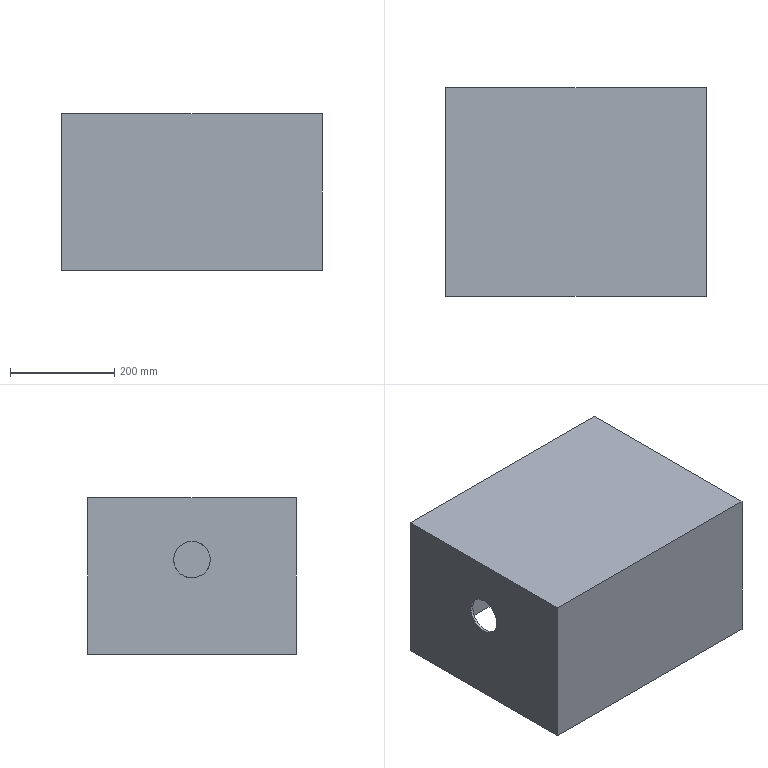Part | NX | features DATUM_CSYS 2, BLOCK 1, EXTRUDE 1, SHELL 1, SKETCH 1 | 1 solid | 12 faces | box 500 x 400 x 300 mm | volume 3606133 mm3 | plane 11 | cylinder 1 | commonest cylinder face diameters 70.226 x1
STEP:
#1=CARTESIAN_POINT('',(500.,0.,0.));
#2=VERTEX_POINT('',#1);
#3=CARTESIAN_POINT('',(500.,400.,0.));
#4=VERTEX_POINT('',#3);
#5=CARTESIAN_POINT('',(500.,200.,0.));
#6=DIRECTION('',(0.,1.,0.));
#7=VECTOR('',#6,1000.);
#8=LINE('',#5,#7);
#9=EDGE_CURVE('',#2,#4,#8,.T.);
#10=ORIENTED_EDGE('',*,*,#9,.F.);
#11=CARTESIAN_POINT('',(0.,0.,0.));
#12=VERTEX_POINT('',#11);
#13=CARTESIAN_POINT('',(250.,0.,0.));
#14=DIRECTION('',(1.,0.,0.));
#15=VECTOR('',#14,1000.);
#16=LINE('',#13,#15);
#17=EDGE_CURVE('',#12,#2,#16,.T.);
#18=ORIENTED_EDGE('',*,*,#17,.F.);
#19=CARTESIAN_POINT('',(0.,400.,0.));
#20=VERTEX_POINT('',#19);
#21=CARTESIAN_POINT('',(0.,200.,0.));
#22=DIRECTION('',(0.,-1.,0.));
#23=VECTOR('',#22,1000.);
#24=LINE('',#21,#23);
#25=EDGE_CURVE('',#20,#12,#24,.T.);
#26=ORIENTED_EDGE('',*,*,#25,.F.);
#27=CARTESIAN_POINT('',(250.,400.,0.));
#28=DIRECTION('',(-1.,0.,0.));
#29=VECTOR('',#28,1000.);
#30=LINE('',#27,#29);
#31=EDGE_CURVE('',#4,#20,#30,.T.);
#32=ORIENTED_EDGE('',*,*,#31,.F.);
#33=EDGE_LOOP('',(#10,#18,#26,#32));
#34=FACE_BOUND('',#33,.T.);
#35=CARTESIAN_POINT('',(5.,5.,0.));
#36=VERTEX_POINT('',#35);
#37=CARTESIAN_POINT('',(495.,5.,0.));
#38=VERTEX_POINT('',#37);
#39=CARTESIAN_POINT('',(250.,5.,0.));
#40=DIRECTION('',(1.,0.,0.));
#41=VECTOR('',#40,1000.);
#42=LINE('',#39,#41);
#43=EDGE_CURVE('',#36,#38,#42,.T.);
#44=ORIENTED_EDGE('',*,*,#43,.T.);
#45=CARTESIAN_POINT('',(495.,395.,0.));
#46=VERTEX_POINT('',#45);
#47=CARTESIAN_POINT('',(495.,200.,0.));
#48=DIRECTION('',(0.,1.,0.));
#49=VECTOR('',#48,1000.);
#50=LINE('',#47,#49);
#51=EDGE_CURVE('',#38,#46,#50,.T.);
#52=ORIENTED_EDGE('',*,*,#51,.T.);
#53=CARTESIAN_POINT('',(5.,395.,0.));
#54=VERTEX_POINT('',#53);
#55=CARTESIAN_POINT('',(250.,395.,0.));
#56=DIRECTION('',(-1.,0.,0.));
#57=VECTOR('',#56,1000.);
#58=LINE('',#55,#57);
#59=EDGE_CURVE('',#46,#54,#58,.T.);
#60=ORIENTED_EDGE('',*,*,#59,.T.);
#61=CARTESIAN_POINT('',(5.,200.,0.));
#62=DIRECTION('',(0.,-1.,0.));
#63=VECTOR('',#62,1000.);
#64=LINE('',#61,#63);
#65=EDGE_CURVE('',#54,#36,#64,.T.);
#66=ORIENTED_EDGE('',*,*,#65,.T.);
#67=EDGE_LOOP('',(#44,#52,#60,#66));
#68=FACE_BOUND('',#67,.T.);
#69=CARTESIAN_POINT('',(250.,200.,0.));
#70=DIRECTION('',(0.,0.,-1.));
#71=DIRECTION('',(-1.,0.,0.));
#72=AXIS2_PLACEMENT_3D('',#69,#70,#71);
#73=PLANE('',#72);
#74=ADVANCED_FACE('',(#34,#68),#73,.T.);
#75=CARTESIAN_POINT('',(500.,0.,300.));
#76=VERTEX_POINT('',#75);
#77=CARTESIAN_POINT('',(0.,0.,300.));
#78=VERTEX_POINT('',#77);
#79=CARTESIAN_POINT('',(250.,0.,300.));
#80=DIRECTION('',(-1.,0.,0.));
#81=VECTOR('',#80,1000.);
#82=LINE('',#79,#81);
#83=EDGE_CURVE('',#76,#78,#82,.T.);
#84=ORIENTED_EDGE('',*,*,#83,.F.);
#85=CARTESIAN_POINT('',(500.,400.,300.));
#86=VERTEX_POINT('',#85);
#87=CARTESIAN_POINT('',(500.,200.,300.));
#88=DIRECTION('',(0.,-1.,0.));
#89=VECTOR('',#88,1000.);
#90=LINE('',#87,#89);
#91=EDGE_CURVE('',#86,#76,#90,.T.);
#92=ORIENTED_EDGE('',*,*,#91,.F.);
#93=CARTESIAN_POINT('',(0.,400.,300.));
#94=VERTEX_POINT('',#93);
#95=CARTESIAN_POINT('',(250.,400.,300.));
#96=DIRECTION('',(1.,0.,0.));
#97=VECTOR('',#96,1000.);
#98=LINE('',#95,#97);
#99=EDGE_CURVE('',#94,#86,#98,.T.);
#100=ORIENTED_EDGE('',*,*,#99,.F.);
#101=CARTESIAN_POINT('',(0.,200.,300.));
#102=DIRECTION('',(0.,1.,0.));
#103=VECTOR('',#102,1000.);
#104=LINE('',#101,#103);
#105=EDGE_CURVE('',#78,#94,#104,.T.);
#106=ORIENTED_EDGE('',*,*,#105,.F.);
#107=EDGE_LOOP('',(#84,#92,#100,#106));
#108=FACE_BOUND('',#107,.T.);
#109=CARTESIAN_POINT('',(250.,200.,300.));
#110=DIRECTION('',(0.,0.,1.));
#111=DIRECTION('',(1.,0.,0.));
#112=AXIS2_PLACEMENT_3D('',#109,#110,#111);
#113=PLANE('',#112);
#114=ADVANCED_FACE('',(#108),#113,.T.);
#115=CARTESIAN_POINT('',(500.,0.,0.));
#116=DIRECTION('',(0.,0.,1.));
#117=VECTOR('',#116,1000.);
#118=LINE('',#115,#117);
#119=EDGE_CURVE('',#2,#76,#118,.T.);
#120=ORIENTED_EDGE('',*,*,#119,.T.);
#121=ORIENTED_EDGE('',*,*,#83,.T.);
#122=CARTESIAN_POINT('',(0.,0.,0.));
#123=DIRECTION('',(0.,0.,1.));
#124=VECTOR('',#123,1000.);
#125=LINE('',#122,#124);
#126=EDGE_CURVE('',#12,#78,#125,.T.);
#127=ORIENTED_EDGE('',*,*,#126,.F.);
#128=ORIENTED_EDGE('',*,*,#17,.T.);
#129=EDGE_LOOP('',(#120,#121,#127,#128));
#130=FACE_BOUND('',#129,.T.);
#131=CARTESIAN_POINT('',(250.,0.,0.));
#132=DIRECTION('',(0.,-1.,0.));
#133=DIRECTION('',(0.,0.,-1.));
#134=AXIS2_PLACEMENT_3D('',#131,#132,#133);
#135=PLANE('',#134);
#136=ADVANCED_FACE('',(#130),#135,.T.);
#137=CARTESIAN_POINT('',(0.,164.887,181.333));
#138=VERTEX_POINT('',#137);
#139=CARTESIAN_POINT('',(0.,200.,181.333));
#140=DIRECTION('',(-1.,0.,0.));
#141=DIRECTION('',(0.,-1.,0.));
#142=AXIS2_PLACEMENT_3D('',#139,#140,#141);
#143=CIRCLE('',#142,35.113);
#144=EDGE_CURVE('',#138,#138,#143,.T.);
#145=ORIENTED_EDGE('',*,*,#144,.F.);
#146=EDGE_LOOP('',(#145));
#147=FACE_BOUND('',#146,.T.);
#148=ORIENTED_EDGE('',*,*,#126,.T.);
#149=ORIENTED_EDGE('',*,*,#105,.T.);
#150=CARTESIAN_POINT('',(0.,400.,0.));
#151=DIRECTION('',(0.,0.,1.));
#152=VECTOR('',#151,1000.);
#153=LINE('',#150,#152);
#154=EDGE_CURVE('',#20,#94,#153,.T.);
#155=ORIENTED_EDGE('',*,*,#154,.F.);
#156=ORIENTED_EDGE('',*,*,#25,.T.);
#157=EDGE_LOOP('',(#148,#149,#155,#156));
#158=FACE_BOUND('',#157,.T.);
#159=CARTESIAN_POINT('',(0.,200.,0.));
#160=DIRECTION('',(-1.,0.,0.));
#161=DIRECTION('',(0.,0.,1.));
#162=AXIS2_PLACEMENT_3D('',#159,#160,#161);
#163=PLANE('',#162);
#164=ADVANCED_FACE('',(#147,#158),#163,.T.);
#165=ORIENTED_EDGE('',*,*,#154,.T.);
#166=ORIENTED_EDGE('',*,*,#99,.T.);
#167=CARTESIAN_POINT('',(500.,400.,0.));
#168=DIRECTION('',(0.,0.,1.));
#169=VECTOR('',#168,1000.);
#170=LINE('',#167,#169);
#171=EDGE_CURVE('',#4,#86,#170,.T.);
#172=ORIENTED_EDGE('',*,*,#171,.F.);
#173=ORIENTED_EDGE('',*,*,#31,.T.);
#174=EDGE_LOOP('',(#165,#166,#172,#173));
#175=FACE_BOUND('',#174,.T.);
#176=CARTESIAN_POINT('',(250.,400.,0.));
#177=DIRECTION('',(0.,1.,0.));
#178=DIRECTION('',(0.,0.,1.));
#179=AXIS2_PLACEMENT_3D('',#176,#177,#178);
#180=PLANE('',#179);
#181=ADVANCED_FACE('',(#175),#180,.T.);
#182=ORIENTED_EDGE('',*,*,#9,.T.);
#183=ORIENTED_EDGE('',*,*,#171,.T.);
#184=ORIENTED_EDGE('',*,*,#91,.T.);
#185=ORIENTED_EDGE('',*,*,#119,.F.);
#186=EDGE_LOOP('',(#182,#183,#184,#185));
#187=FACE_BOUND('',#186,.T.);
#188=CARTESIAN_POINT('',(500.,200.,0.));
#189=DIRECTION('',(1.,0.,0.));
#190=DIRECTION('',(0.,0.,-1.));
#191=AXIS2_PLACEMENT_3D('',#188,#189,#190);
#192=PLANE('',#191);
#193=ADVANCED_FACE('',(#187),#192,.T.);
#194=CARTESIAN_POINT('',(495.,5.,295.));
#195=VERTEX_POINT('',#194);
#196=CARTESIAN_POINT('',(5.,5.,295.));
#197=VERTEX_POINT('',#196);
#198=CARTESIAN_POINT('',(250.,5.,295.));
#199=DIRECTION('',(-1.,0.,0.));
#200=VECTOR('',#199,1000.);
#201=LINE('',#198,#200);
#202=EDGE_CURVE('',#195,#197,#201,.T.);
#203=ORIENTED_EDGE('',*,*,#202,.T.);
#204=CARTESIAN_POINT('',(5.,395.,295.));
#205=VERTEX_POINT('',#204);
#206=CARTESIAN_POINT('',(5.,200.,295.));
#207=DIRECTION('',(0.,1.,0.));
#208=VECTOR('',#207,1000.);
#209=LINE('',#206,#208);
#210=EDGE_CURVE('',#197,#205,#209,.T.);
#211=ORIENTED_EDGE('',*,*,#210,.T.);
#212=CARTESIAN_POINT('',(495.,395.,295.));
#213=VERTEX_POINT('',#212);
#214=CARTESIAN_POINT('',(250.,395.,295.));
#215=DIRECTION('',(1.,0.,0.));
#216=VECTOR('',#215,1000.);
#217=LINE('',#214,#216);
#218=EDGE_CURVE('',#205,#213,#217,.T.);
#219=ORIENTED_EDGE('',*,*,#218,.T.);
#220=CARTESIAN_POINT('',(495.,200.,295.));
#221=DIRECTION('',(0.,-1.,0.));
#222=VECTOR('',#221,1000.);
#223=LINE('',#220,#222);
#224=EDGE_CURVE('',#213,#195,#223,.T.);
#225=ORIENTED_EDGE('',*,*,#224,.T.);
#226=EDGE_LOOP('',(#203,#211,#219,#225));
#227=FACE_BOUND('',#226,.T.);
#228=CARTESIAN_POINT('',(250.,200.,295.));
#229=DIRECTION('',(0.,0.,1.));
#230=DIRECTION('',(1.,0.,0.));
#231=AXIS2_PLACEMENT_3D('',#228,#229,#230);
#232=PLANE('',#231);
#233=ADVANCED_FACE('',(#227),#232,.F.);
#234=CARTESIAN_POINT('',(495.,5.,0.));
#235=DIRECTION('',(0.,0.,1.));
#236=VECTOR('',#235,1000.);
#237=LINE('',#234,#236);
#238=EDGE_CURVE('',#38,#195,#237,.T.);
#239=ORIENTED_EDGE('',*,*,#238,.F.);
#240=ORIENTED_EDGE('',*,*,#43,.F.);
#241=CARTESIAN_POINT('',(5.,5.,0.));
#242=DIRECTION('',(0.,0.,1.));
#243=VECTOR('',#242,1000.);
#244=LINE('',#241,#243);
#245=EDGE_CURVE('',#36,#197,#244,.T.);
#246=ORIENTED_EDGE('',*,*,#245,.T.);
#247=ORIENTED_EDGE('',*,*,#202,.F.);
#248=EDGE_LOOP('',(#239,#240,#246,#247));
#249=FACE_BOUND('',#248,.T.);
#250=CARTESIAN_POINT('',(250.,5.,0.));
#251=DIRECTION('',(0.,-1.,0.));
#252=DIRECTION('',(0.,0.,-1.));
#253=AXIS2_PLACEMENT_3D('',#250,#251,#252);
#254=PLANE('',#253);
#255=ADVANCED_FACE('',(#249),#254,.F.);
#256=CARTESIAN_POINT('',(5.,200.,216.446));
#257=VERTEX_POINT('',#256);
#258=CARTESIAN_POINT('',(5.,200.,181.333));
#259=DIRECTION('',(-1.,0.,0.));
#260=DIRECTION('',(0.,0.,1.));
#261=AXIS2_PLACEMENT_3D('',#258,#259,#260);
#262=CIRCLE('',#261,35.113);
#263=EDGE_CURVE('',#257,#257,#262,.T.);
#264=ORIENTED_EDGE('',*,*,#263,.T.);
#265=EDGE_LOOP('',(#264));
#266=FACE_BOUND('',#265,.T.);
#267=ORIENTED_EDGE('',*,*,#245,.F.);
#268=ORIENTED_EDGE('',*,*,#65,.F.);
#269=CARTESIAN_POINT('',(5.,395.,0.));
#270=DIRECTION('',(0.,0.,1.));
#271=VECTOR('',#270,1000.);
#272=LINE('',#269,#271);
#273=EDGE_CURVE('',#54,#205,#272,.T.);
#274=ORIENTED_EDGE('',*,*,#273,.T.);
#275=ORIENTED_EDGE('',*,*,#210,.F.);
#276=EDGE_LOOP('',(#267,#268,#274,#275));
#277=FACE_BOUND('',#276,.T.);
#278=CARTESIAN_POINT('',(5.,200.,0.));
#279=DIRECTION('',(-1.,0.,0.));
#280=DIRECTION('',(0.,0.,1.));
#281=AXIS2_PLACEMENT_3D('',#278,#279,#280);
#282=PLANE('',#281);
#283=ADVANCED_FACE('',(#266,#277),#282,.F.);
#284=ORIENTED_EDGE('',*,*,#273,.F.);
#285=ORIENTED_EDGE('',*,*,#59,.F.);
#286=CARTESIAN_POINT('',(495.,395.,0.));
#287=DIRECTION('',(0.,0.,1.));
#288=VECTOR('',#287,1000.);
#289=LINE('',#286,#288);
#290=EDGE_CURVE('',#46,#213,#289,.T.);
#291=ORIENTED_EDGE('',*,*,#290,.T.);
#292=ORIENTED_EDGE('',*,*,#218,.F.);
#293=EDGE_LOOP('',(#284,#285,#291,#292));
#294=FACE_BOUND('',#293,.T.);
#295=CARTESIAN_POINT('',(250.,395.,0.));
#296=DIRECTION('',(0.,1.,0.));
#297=DIRECTION('',(0.,0.,1.));
#298=AXIS2_PLACEMENT_3D('',#295,#296,#297);
#299=PLANE('',#298);
#300=ADVANCED_FACE('',(#294),#299,.F.);
#301=ORIENTED_EDGE('',*,*,#51,.F.);
#302=ORIENTED_EDGE('',*,*,#238,.T.);
#303=ORIENTED_EDGE('',*,*,#224,.F.);
#304=ORIENTED_EDGE('',*,*,#290,.F.);
#305=EDGE_LOOP('',(#301,#302,#303,#304));
#306=FACE_BOUND('',#305,.T.);
#307=CARTESIAN_POINT('',(495.,200.,0.));
#308=DIRECTION('',(1.,0.,0.));
#309=DIRECTION('',(0.,0.,-1.));
#310=AXIS2_PLACEMENT_3D('',#307,#308,#309);
#311=PLANE('',#310);
#312=ADVANCED_FACE('',(#306),#311,.F.);
#313=ORIENTED_EDGE('',*,*,#144,.T.);
#314=EDGE_LOOP('',(#313));
#315=FACE_BOUND('',#314,.T.);
#316=ORIENTED_EDGE('',*,*,#263,.F.);
#317=EDGE_LOOP('',(#316));
#318=FACE_BOUND('',#317,.T.);
#319=CARTESIAN_POINT('',(41.,200.,181.333));
#320=DIRECTION('',(-1.,0.,0.));
#321=DIRECTION('',(0.,0.,1.));
#322=AXIS2_PLACEMENT_3D('',#319,#320,#321);
#323=CYLINDRICAL_SURFACE('',#322,35.113);
#324=ADVANCED_FACE('',(#315,#318),#323,.F.);
#325=CLOSED_SHELL('',(#74,#114,#136,#164,#181,#193,#233,#255,#283,#300,#312,#324));
#326=MANIFOLD_SOLID_BREP('',#325);
#327=(LENGTH_UNIT()NAMED_UNIT(*)SI_UNIT(.MILLI.,.METRE.));
#328=UNCERTAINTY_MEASURE_WITH_UNIT(LENGTH_MEASURE(0.00001),#327,'','');
#329=(NAMED_UNIT(*)PLANE_ANGLE_UNIT()SI_UNIT($,.RADIAN.));
#330=(NAMED_UNIT(*)SI_UNIT($,.STERADIAN.)SOLID_ANGLE_UNIT());
#331=(GEOMETRIC_REPRESENTATION_CONTEXT(3)GLOBAL_UNCERTAINTY_ASSIGNED_CONTEXT((#328))GLOBAL_UNIT_ASSIGNED_CONTEXT((#327,#329,#330))REPRESENTATION_CONTEXT('',''));
#332=ADVANCED_BREP_SHAPE_REPRESENTATION('',(#326),#331);